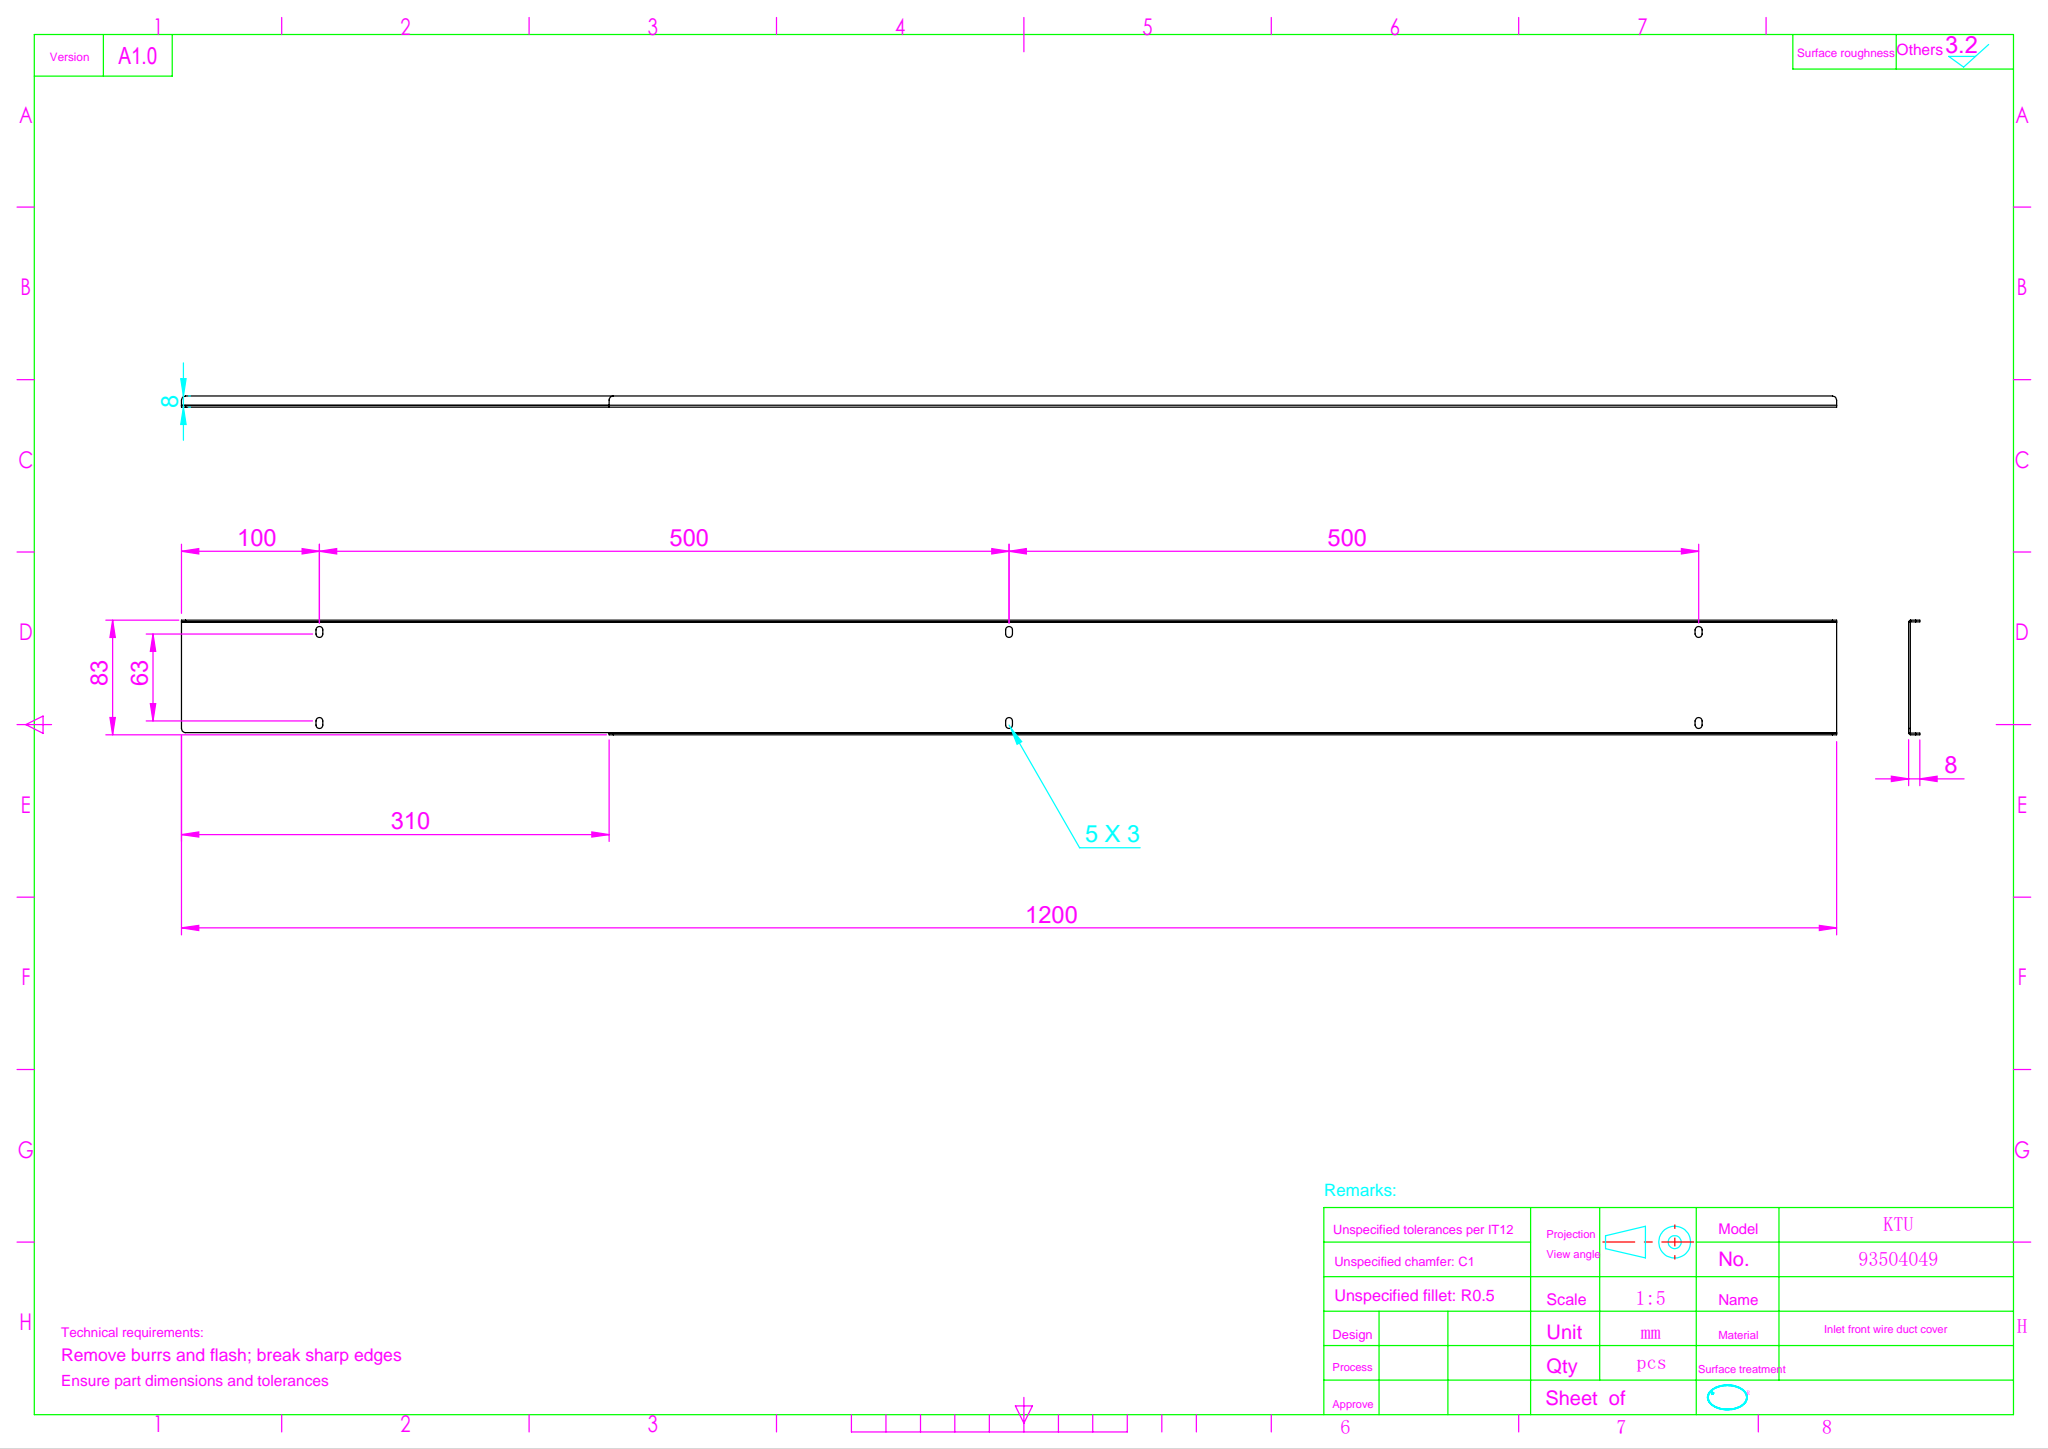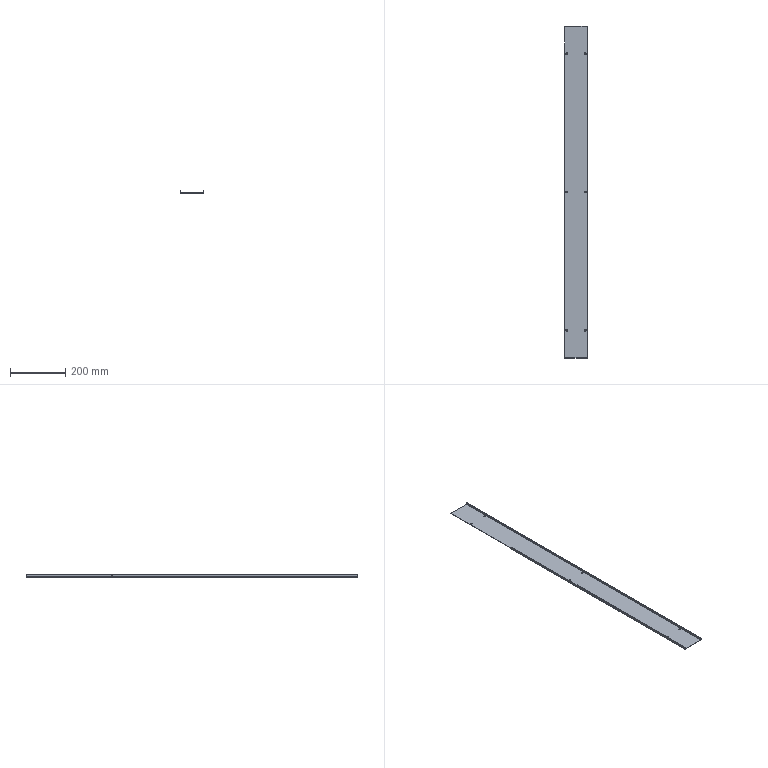Part | SolidWorks | features EdgeFlange 2, ICE 2, Fillet 1, FlatPattern 1, LPattern 1, SMBaseFlange 1, SheetMetal 1 | 1 solid | 57 faces | box 83 x 1200 x 8 mm | volume 134894 mm3 | plane 30 | cylinder 27 | commonest cylinder face diameters 5 x18 6 x5 0.4 x2 2.8 x2